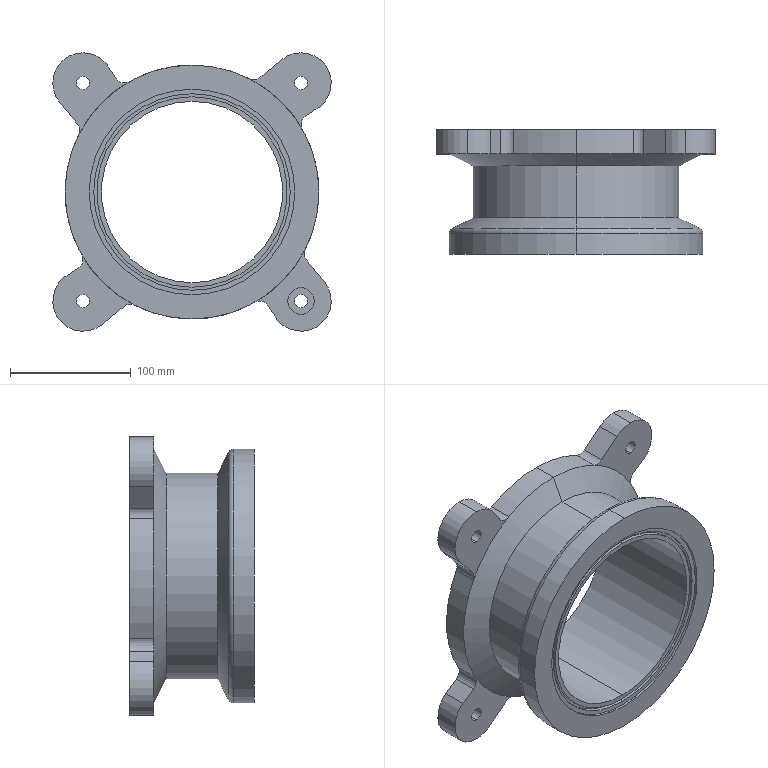Part | SolidWorks | features ICE 5, CirPattern 2, Revolution 1 | 1 solid | 106 faces | box 230.312 x 103 x 230.312 mm | volume 1234015 mm3 | cylinder 69 | plane 31 | cone 4 | torus 2 | commonest cylinder face diameters 10 x20 16 x10 11 x8 210 x7 50 x6 170 x6